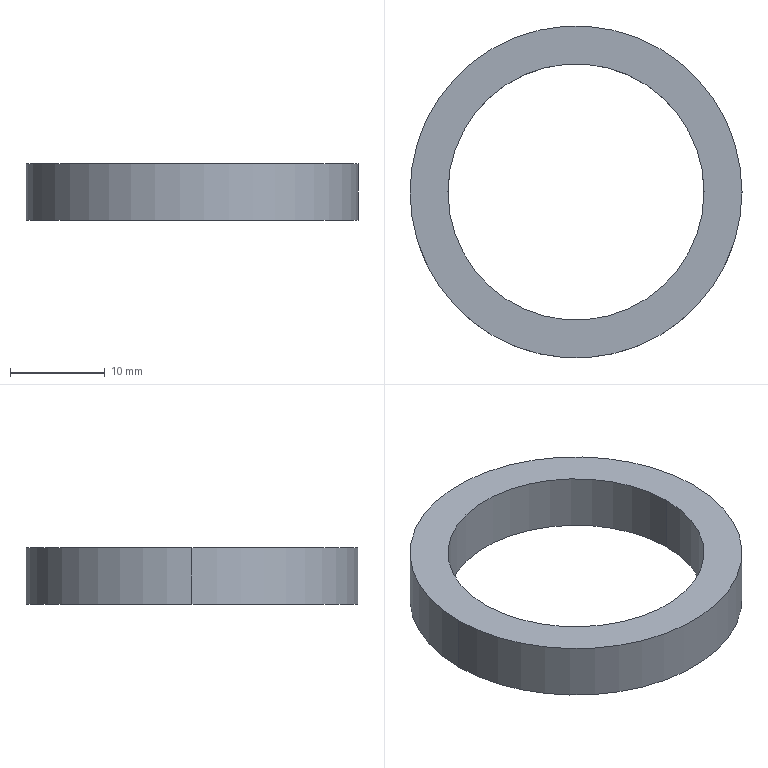Part | SolidWorks | features Extrusion 1 | 1 solid | 6 faces | box 35 x 35 x 6 mm | volume 2337 mm3 | cylinder 4 | plane 2 | commonest cylinder face diameters 27 x2 35 x2
STEP:
#1=CARTESIAN_POINT('',(-13.5,0.,6.));
#2=VERTEX_POINT('',#1);
#3=CARTESIAN_POINT('',(13.5,0.,6.));
#4=VERTEX_POINT('',#3);
#5=CARTESIAN_POINT('',(0.,0.,6.));
#6=DIRECTION('',(0.,0.,1.));
#7=DIRECTION('',(1.,0.,0.));
#8=AXIS2_PLACEMENT_3D('',#5,#6,#7);
#9=CIRCLE('',#8,13.5);
#10=EDGE_CURVE('',#2,#4,#9,.T.);
#11=ORIENTED_EDGE('',*,*,#10,.T.);
#12=CARTESIAN_POINT('',(13.5,0.,0.));
#13=VERTEX_POINT('',#12);
#14=CARTESIAN_POINT('',(13.5,0.,6.));
#15=DIRECTION('',(0.,0.,-1.));
#16=VECTOR('',#15,1000.);
#17=LINE('',#14,#16);
#18=EDGE_CURVE('',#4,#13,#17,.T.);
#19=ORIENTED_EDGE('',*,*,#18,.T.);
#20=CARTESIAN_POINT('',(-13.5,0.,0.));
#21=VERTEX_POINT('',#20);
#22=CARTESIAN_POINT('',(0.,0.,0.));
#23=DIRECTION('',(0.,0.,1.));
#24=DIRECTION('',(1.,0.,0.));
#25=AXIS2_PLACEMENT_3D('',#22,#23,#24);
#26=CIRCLE('',#25,13.5);
#27=EDGE_CURVE('',#21,#13,#26,.T.);
#28=ORIENTED_EDGE('',*,*,#27,.F.);
#29=CARTESIAN_POINT('',(-13.5,0.,6.));
#30=DIRECTION('',(0.,0.,-1.));
#31=VECTOR('',#30,1000.);
#32=LINE('',#29,#31);
#33=EDGE_CURVE('',#2,#21,#32,.T.);
#34=ORIENTED_EDGE('',*,*,#33,.F.);
#35=EDGE_LOOP('',(#11,#19,#28,#34));
#36=FACE_OUTER_BOUND('',#35,.T.);
#37=CARTESIAN_POINT('',(0.,0.,6.));
#38=DIRECTION('',(0.,0.,-1.));
#39=DIRECTION('',(-1.,0.,0.));
#40=AXIS2_PLACEMENT_3D('',#37,#38,#39);
#41=CYLINDRICAL_SURFACE('',#40,13.5);
#42=ADVANCED_FACE('',(#36),#41,.F.);
#43=CARTESIAN_POINT('',(17.5,0.,6.));
#44=VERTEX_POINT('',#43);
#45=CARTESIAN_POINT('',(-17.5,0.,6.));
#46=VERTEX_POINT('',#45);
#47=CARTESIAN_POINT('',(0.,0.,6.));
#48=DIRECTION('',(0.,0.,1.));
#49=DIRECTION('',(1.,0.,0.));
#50=AXIS2_PLACEMENT_3D('',#47,#48,#49);
#51=CIRCLE('',#50,17.5);
#52=EDGE_CURVE('',#44,#46,#51,.T.);
#53=ORIENTED_EDGE('',*,*,#52,.F.);
#54=CARTESIAN_POINT('',(17.5,0.,0.));
#55=VERTEX_POINT('',#54);
#56=CARTESIAN_POINT('',(17.5,0.,6.));
#57=DIRECTION('',(0.,0.,-1.));
#58=VECTOR('',#57,1000.);
#59=LINE('',#56,#58);
#60=EDGE_CURVE('',#44,#55,#59,.T.);
#61=ORIENTED_EDGE('',*,*,#60,.T.);
#62=CARTESIAN_POINT('',(-17.5,0.,0.));
#63=VERTEX_POINT('',#62);
#64=CARTESIAN_POINT('',(0.,0.,0.));
#65=DIRECTION('',(0.,0.,1.));
#66=DIRECTION('',(1.,0.,0.));
#67=AXIS2_PLACEMENT_3D('',#64,#65,#66);
#68=CIRCLE('',#67,17.5);
#69=EDGE_CURVE('',#55,#63,#68,.T.);
#70=ORIENTED_EDGE('',*,*,#69,.T.);
#71=CARTESIAN_POINT('',(-17.5,0.,6.));
#72=DIRECTION('',(0.,0.,-1.));
#73=VECTOR('',#72,1000.);
#74=LINE('',#71,#73);
#75=EDGE_CURVE('',#46,#63,#74,.T.);
#76=ORIENTED_EDGE('',*,*,#75,.F.);
#77=EDGE_LOOP('',(#53,#61,#70,#76));
#78=FACE_OUTER_BOUND('',#77,.T.);
#79=CARTESIAN_POINT('',(0.,0.,6.));
#80=DIRECTION('',(0.,0.,-1.));
#81=DIRECTION('',(-1.,0.,0.));
#82=AXIS2_PLACEMENT_3D('',#79,#80,#81);
#83=CYLINDRICAL_SURFACE('',#82,17.5);
#84=ADVANCED_FACE('',(#78),#83,.T.);
#85=CARTESIAN_POINT('',(0.,0.,6.));
#86=DIRECTION('',(0.,0.,1.));
#87=DIRECTION('',(1.,0.,0.));
#88=AXIS2_PLACEMENT_3D('',#85,#86,#87);
#89=CIRCLE('',#88,17.5);
#90=EDGE_CURVE('',#46,#44,#89,.T.);
#91=ORIENTED_EDGE('',*,*,#90,.T.);
#92=ORIENTED_EDGE('',*,*,#52,.T.);
#93=EDGE_LOOP('',(#91,#92));
#94=FACE_OUTER_BOUND('',#93,.T.);
#95=ORIENTED_EDGE('',*,*,#10,.F.);
#96=CARTESIAN_POINT('',(0.,0.,6.));
#97=DIRECTION('',(0.,0.,1.));
#98=DIRECTION('',(1.,0.,0.));
#99=AXIS2_PLACEMENT_3D('',#96,#97,#98);
#100=CIRCLE('',#99,13.5);
#101=EDGE_CURVE('',#4,#2,#100,.T.);
#102=ORIENTED_EDGE('',*,*,#101,.F.);
#103=EDGE_LOOP('',(#95,#102));
#104=FACE_BOUND('',#103,.T.);
#105=CARTESIAN_POINT('',(0.,0.,6.));
#106=DIRECTION('',(0.,0.,1.));
#107=DIRECTION('',(1.,0.,0.));
#108=AXIS2_PLACEMENT_3D('',#105,#106,#107);
#109=PLANE('',#108);
#110=ADVANCED_FACE('',(#94,#104),#109,.T.);
#111=CARTESIAN_POINT('',(0.,0.,0.));
#112=DIRECTION('',(0.,0.,1.));
#113=DIRECTION('',(1.,0.,0.));
#114=AXIS2_PLACEMENT_3D('',#111,#112,#113);
#115=CIRCLE('',#114,17.5);
#116=EDGE_CURVE('',#63,#55,#115,.T.);
#117=ORIENTED_EDGE('',*,*,#116,.F.);
#118=ORIENTED_EDGE('',*,*,#69,.F.);
#119=EDGE_LOOP('',(#117,#118));
#120=FACE_OUTER_BOUND('',#119,.T.);
#121=ORIENTED_EDGE('',*,*,#27,.T.);
#122=CARTESIAN_POINT('',(0.,0.,0.));
#123=DIRECTION('',(0.,0.,1.));
#124=DIRECTION('',(1.,0.,0.));
#125=AXIS2_PLACEMENT_3D('',#122,#123,#124);
#126=CIRCLE('',#125,13.5);
#127=EDGE_CURVE('',#13,#21,#126,.T.);
#128=ORIENTED_EDGE('',*,*,#127,.T.);
#129=EDGE_LOOP('',(#121,#128));
#130=FACE_BOUND('',#129,.T.);
#131=CARTESIAN_POINT('',(0.,0.,0.));
#132=DIRECTION('',(0.,0.,1.));
#133=DIRECTION('',(1.,0.,0.));
#134=AXIS2_PLACEMENT_3D('',#131,#132,#133);
#135=PLANE('',#134);
#136=ADVANCED_FACE('',(#120,#130),#135,.F.);
#137=ORIENTED_EDGE('',*,*,#60,.F.);
#138=ORIENTED_EDGE('',*,*,#90,.F.);
#139=ORIENTED_EDGE('',*,*,#75,.T.);
#140=ORIENTED_EDGE('',*,*,#116,.T.);
#141=EDGE_LOOP('',(#137,#138,#139,#140));
#142=FACE_OUTER_BOUND('',#141,.T.);
#143=CARTESIAN_POINT('',(0.,0.,6.));
#144=DIRECTION('',(0.,0.,-1.));
#145=DIRECTION('',(-1.,0.,0.));
#146=AXIS2_PLACEMENT_3D('',#143,#144,#145);
#147=CYLINDRICAL_SURFACE('',#146,17.5);
#148=ADVANCED_FACE('',(#142),#147,.T.);
#149=ORIENTED_EDGE('',*,*,#18,.F.);
#150=ORIENTED_EDGE('',*,*,#101,.T.);
#151=ORIENTED_EDGE('',*,*,#33,.T.);
#152=ORIENTED_EDGE('',*,*,#127,.F.);
#153=EDGE_LOOP('',(#149,#150,#151,#152));
#154=FACE_OUTER_BOUND('',#153,.T.);
#155=CARTESIAN_POINT('',(0.,0.,6.));
#156=DIRECTION('',(0.,0.,-1.));
#157=DIRECTION('',(-1.,0.,0.));
#158=AXIS2_PLACEMENT_3D('',#155,#156,#157);
#159=CYLINDRICAL_SURFACE('',#158,13.5);
#160=ADVANCED_FACE('',(#154),#159,.F.);
#161=CLOSED_SHELL('',(#42,#84,#110,#136,#148,#160));
#162=MANIFOLD_SOLID_BREP('',#161);
#163=CARTESIAN_POINT('',(0.,0.,0.));
#164=DIRECTION('',(0.,0.,1.));
#165=DIRECTION('',(1.,0.,0.));
#166=AXIS2_PLACEMENT_3D('',#163,#164,#165);
#167=(LENGTH_UNIT()NAMED_UNIT(*)SI_UNIT(.MILLI.,.METRE.));
#168=UNCERTAINTY_MEASURE_WITH_UNIT(LENGTH_MEASURE(0.00001),#167,'','');
#169=(NAMED_UNIT(*)PLANE_ANGLE_UNIT()SI_UNIT($,.RADIAN.));
#170=(NAMED_UNIT(*)SI_UNIT($,.STERADIAN.)SOLID_ANGLE_UNIT());
#171=(GEOMETRIC_REPRESENTATION_CONTEXT(3)GLOBAL_UNCERTAINTY_ASSIGNED_CONTEXT((#168))GLOBAL_UNIT_ASSIGNED_CONTEXT((#167,#169,#170))REPRESENTATION_CONTEXT('',''));
#172=ADVANCED_BREP_SHAPE_REPRESENTATION('',(#162,#166),#171);